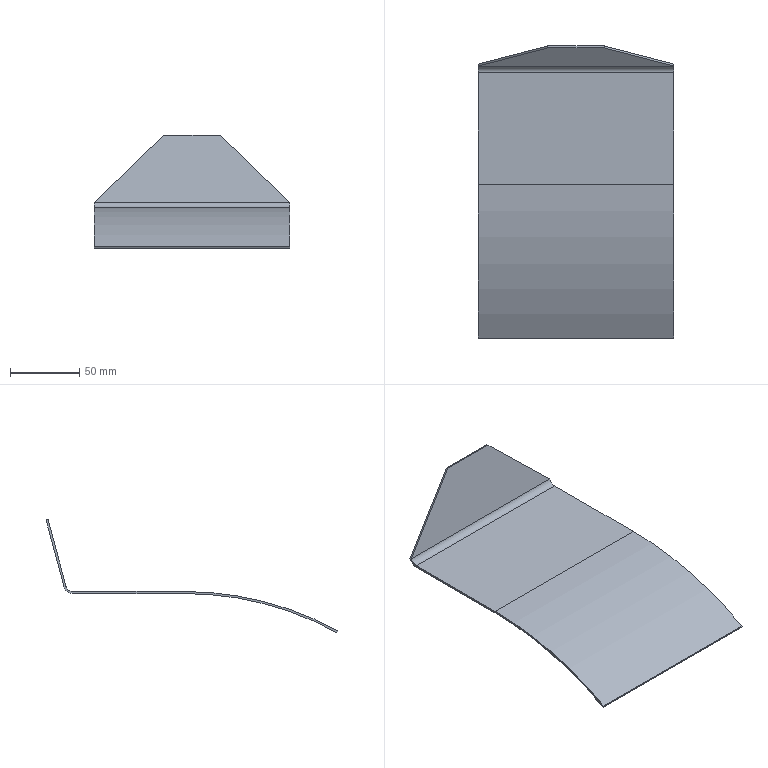Part | SolidWorks | features Chamfer 1, Extrusion 1 | 1 solid | 14 faces | box 141 x 210.455 x 81.673 mm | volume 49794 mm3 | plane 10 | cylinder 4 | commonest cylinder face diameters 10 x1 13 x1 458.6 x1 461.6 x1
STEP:
#1=CARTESIAN_POINT('',(-70.5,80.4,230.8));
#2=VERTEX_POINT('',#1);
#3=CARTESIAN_POINT('',(-70.5,85.23,234.506));
#4=VERTEX_POINT('',#3);
#5=CARTESIAN_POINT('',(-70.5,80.4,235.8));
#6=DIRECTION('',(1.,0.,0.));
#7=DIRECTION('',(0.,0.,-1.));
#8=AXIS2_PLACEMENT_3D('',#5,#6,#7);
#9=CIRCLE('',#8,5.);
#10=EDGE_CURVE('',#2,#4,#9,.T.);
#11=ORIENTED_EDGE('',*,*,#10,.F.);
#12=CARTESIAN_POINT('',(70.5,80.4,230.8));
#13=VERTEX_POINT('',#12);
#14=CARTESIAN_POINT('',(70.5,80.4,230.8));
#15=DIRECTION('',(-1.,0.,0.));
#16=VECTOR('',#15,1000.);
#17=LINE('',#14,#16);
#18=EDGE_CURVE('',#13,#2,#17,.T.);
#19=ORIENTED_EDGE('',*,*,#18,.F.);
#20=CARTESIAN_POINT('',(70.5,85.23,234.506));
#21=VERTEX_POINT('',#20);
#22=CARTESIAN_POINT('',(70.5,80.4,235.8));
#23=DIRECTION('',(1.,0.,0.));
#24=DIRECTION('',(0.,0.,-1.));
#25=AXIS2_PLACEMENT_3D('',#22,#23,#24);
#26=CIRCLE('',#25,5.);
#27=EDGE_CURVE('',#13,#21,#26,.T.);
#28=ORIENTED_EDGE('',*,*,#27,.T.);
#29=CARTESIAN_POINT('',(70.5,85.23,234.506));
#30=DIRECTION('',(-1.,0.,0.));
#31=VECTOR('',#30,1000.);
#32=LINE('',#29,#31);
#33=EDGE_CURVE('',#21,#4,#32,.T.);
#34=ORIENTED_EDGE('',*,*,#33,.T.);
#35=EDGE_LOOP('',(#11,#19,#28,#34));
#36=FACE_OUTER_BOUND('',#35,.T.);
#37=CARTESIAN_POINT('',(70.5,80.4,235.8));
#38=DIRECTION('',(-1.,0.,0.));
#39=DIRECTION('',(0.,0.,1.));
#40=AXIS2_PLACEMENT_3D('',#37,#38,#39);
#41=CYLINDRICAL_SURFACE('',#40,5.);
#42=ADVANCED_FACE('',(#36),#41,.F.);
#43=CARTESIAN_POINT('',(-70.5,0.,230.8));
#44=VERTEX_POINT('',#43);
#45=CARTESIAN_POINT('',(-70.5,0.,230.8));
#46=DIRECTION('',(0.,-1.,0.));
#47=VECTOR('',#46,1000.);
#48=LINE('',#45,#47);
#49=EDGE_CURVE('',#2,#44,#48,.T.);
#50=ORIENTED_EDGE('',*,*,#49,.T.);
#51=CARTESIAN_POINT('',(70.5,0.,230.8));
#52=VERTEX_POINT('',#51);
#53=CARTESIAN_POINT('',(70.5,0.,230.8));
#54=DIRECTION('',(-1.,0.,0.));
#55=VECTOR('',#54,1000.);
#56=LINE('',#53,#55);
#57=EDGE_CURVE('',#52,#44,#56,.T.);
#58=ORIENTED_EDGE('',*,*,#57,.F.);
#59=CARTESIAN_POINT('',(70.5,0.,230.8));
#60=DIRECTION('',(0.,-1.,0.));
#61=VECTOR('',#60,1000.);
#62=LINE('',#59,#61);
#63=EDGE_CURVE('',#13,#52,#62,.T.);
#64=ORIENTED_EDGE('',*,*,#63,.F.);
#65=ORIENTED_EDGE('',*,*,#18,.T.);
#66=EDGE_LOOP('',(#50,#58,#64,#65));
#67=FACE_OUTER_BOUND('',#66,.T.);
#68=CARTESIAN_POINT('',(70.5,0.,230.8));
#69=DIRECTION('',(0.,0.,-1.));
#70=DIRECTION('',(-1.,0.,0.));
#71=AXIS2_PLACEMENT_3D('',#68,#69,#70);
#72=PLANE('',#71);
#73=ADVANCED_FACE('',(#67),#72,.F.);
#74=CARTESIAN_POINT('',(-70.5,-110.836,202.445));
#75=VERTEX_POINT('',#74);
#76=CARTESIAN_POINT('',(-70.5,0.,0.));
#77=DIRECTION('',(1.,0.,0.));
#78=DIRECTION('',(0.,0.,-1.));
#79=AXIS2_PLACEMENT_3D('',#76,#77,#78);
#80=CIRCLE('',#79,230.8);
#81=EDGE_CURVE('',#44,#75,#80,.T.);
#82=ORIENTED_EDGE('',*,*,#81,.T.);
#83=CARTESIAN_POINT('',(70.5,-110.836,202.445));
#84=VERTEX_POINT('',#83);
#85=CARTESIAN_POINT('',(70.5,-110.836,202.445));
#86=DIRECTION('',(-1.,0.,0.));
#87=VECTOR('',#86,1000.);
#88=LINE('',#85,#87);
#89=EDGE_CURVE('',#84,#75,#88,.T.);
#90=ORIENTED_EDGE('',*,*,#89,.F.);
#91=CARTESIAN_POINT('',(70.5,0.,0.));
#92=DIRECTION('',(1.,0.,0.));
#93=DIRECTION('',(0.,0.,-1.));
#94=AXIS2_PLACEMENT_3D('',#91,#92,#93);
#95=CIRCLE('',#94,230.8);
#96=EDGE_CURVE('',#52,#84,#95,.T.);
#97=ORIENTED_EDGE('',*,*,#96,.F.);
#98=ORIENTED_EDGE('',*,*,#57,.T.);
#99=EDGE_LOOP('',(#82,#90,#97,#98));
#100=FACE_OUTER_BOUND('',#99,.T.);
#101=CARTESIAN_POINT('',(70.5,0.,0.));
#102=DIRECTION('',(-1.,0.,0.));
#103=DIRECTION('',(0.,0.,1.));
#104=AXIS2_PLACEMENT_3D('',#101,#102,#103);
#105=CYLINDRICAL_SURFACE('',#104,230.8);
#106=ADVANCED_FACE('',(#100),#105,.T.);
#107=CARTESIAN_POINT('',(-70.5,-110.115,201.13));
#108=VERTEX_POINT('',#107);
#109=CARTESIAN_POINT('',(-70.5,0.,0.));
#110=DIRECTION('',(0.,-0.4802,0.8771));
#111=VECTOR('',#110,1000.);
#112=LINE('',#109,#111);
#113=EDGE_CURVE('',#108,#75,#112,.T.);
#114=ORIENTED_EDGE('',*,*,#113,.F.);
#115=CARTESIAN_POINT('',(70.5,-110.115,201.13));
#116=VERTEX_POINT('',#115);
#117=CARTESIAN_POINT('',(70.5,-110.115,201.13));
#118=DIRECTION('',(-1.,0.,0.));
#119=VECTOR('',#118,1000.);
#120=LINE('',#117,#119);
#121=EDGE_CURVE('',#116,#108,#120,.T.);
#122=ORIENTED_EDGE('',*,*,#121,.F.);
#123=CARTESIAN_POINT('',(70.5,0.,0.));
#124=DIRECTION('',(0.,-0.4802,0.8771));
#125=VECTOR('',#124,1000.);
#126=LINE('',#123,#125);
#127=EDGE_CURVE('',#116,#84,#126,.T.);
#128=ORIENTED_EDGE('',*,*,#127,.T.);
#129=ORIENTED_EDGE('',*,*,#89,.T.);
#130=EDGE_LOOP('',(#114,#122,#128,#129));
#131=FACE_OUTER_BOUND('',#130,.T.);
#132=CARTESIAN_POINT('',(70.5,0.,0.));
#133=DIRECTION('',(0.,-0.8771,-0.4802));
#134=DIRECTION('',(0.,0.4802,-0.8771));
#135=AXIS2_PLACEMENT_3D('',#132,#133,#134);
#136=PLANE('',#135);
#137=ADVANCED_FACE('',(#131),#136,.T.);
#138=CARTESIAN_POINT('',(-70.5,0.,229.3));
#139=VERTEX_POINT('',#138);
#140=CARTESIAN_POINT('',(-70.5,0.,0.));
#141=DIRECTION('',(1.,0.,0.));
#142=DIRECTION('',(0.,0.,-1.));
#143=AXIS2_PLACEMENT_3D('',#140,#141,#142);
#144=CIRCLE('',#143,229.3);
#145=EDGE_CURVE('',#139,#108,#144,.T.);
#146=ORIENTED_EDGE('',*,*,#145,.F.);
#147=CARTESIAN_POINT('',(70.5,0.,229.3));
#148=VERTEX_POINT('',#147);
#149=CARTESIAN_POINT('',(70.5,0.,229.3));
#150=DIRECTION('',(-1.,0.,0.));
#151=VECTOR('',#150,1000.);
#152=LINE('',#149,#151);
#153=EDGE_CURVE('',#148,#139,#152,.T.);
#154=ORIENTED_EDGE('',*,*,#153,.F.);
#155=CARTESIAN_POINT('',(70.5,0.,0.));
#156=DIRECTION('',(1.,0.,0.));
#157=DIRECTION('',(0.,0.,-1.));
#158=AXIS2_PLACEMENT_3D('',#155,#156,#157);
#159=CIRCLE('',#158,229.3);
#160=EDGE_CURVE('',#148,#116,#159,.T.);
#161=ORIENTED_EDGE('',*,*,#160,.T.);
#162=ORIENTED_EDGE('',*,*,#121,.T.);
#163=EDGE_LOOP('',(#146,#154,#161,#162));
#164=FACE_OUTER_BOUND('',#163,.T.);
#165=CARTESIAN_POINT('',(70.5,0.,0.));
#166=DIRECTION('',(-1.,0.,0.));
#167=DIRECTION('',(0.,0.,1.));
#168=AXIS2_PLACEMENT_3D('',#165,#166,#167);
#169=CYLINDRICAL_SURFACE('',#168,229.3);
#170=ADVANCED_FACE('',(#164),#169,.F.);
#171=CARTESIAN_POINT('',(-70.5,80.4,229.3));
#172=VERTEX_POINT('',#171);
#173=CARTESIAN_POINT('',(-70.5,0.,229.3));
#174=DIRECTION('',(0.,1.,0.));
#175=VECTOR('',#174,1000.);
#176=LINE('',#173,#175);
#177=EDGE_CURVE('',#139,#172,#176,.T.);
#178=ORIENTED_EDGE('',*,*,#177,.T.);
#179=CARTESIAN_POINT('',(70.5,80.4,229.3));
#180=VERTEX_POINT('',#179);
#181=CARTESIAN_POINT('',(70.5,80.4,229.3));
#182=DIRECTION('',(-1.,0.,0.));
#183=VECTOR('',#182,1000.);
#184=LINE('',#181,#183);
#185=EDGE_CURVE('',#180,#172,#184,.T.);
#186=ORIENTED_EDGE('',*,*,#185,.F.);
#187=CARTESIAN_POINT('',(70.5,0.,229.3));
#188=DIRECTION('',(0.,1.,0.));
#189=VECTOR('',#188,1000.);
#190=LINE('',#187,#189);
#191=EDGE_CURVE('',#148,#180,#190,.T.);
#192=ORIENTED_EDGE('',*,*,#191,.F.);
#193=ORIENTED_EDGE('',*,*,#153,.T.);
#194=EDGE_LOOP('',(#178,#186,#192,#193));
#195=FACE_OUTER_BOUND('',#194,.T.);
#196=CARTESIAN_POINT('',(70.5,0.,229.3));
#197=DIRECTION('',(0.,0.,1.));
#198=DIRECTION('',(1.,0.,0.));
#199=AXIS2_PLACEMENT_3D('',#196,#197,#198);
#200=PLANE('',#199);
#201=ADVANCED_FACE('',(#195),#200,.F.);
#202=CARTESIAN_POINT('',(-70.5,86.679,234.118));
#203=VERTEX_POINT('',#202);
#204=CARTESIAN_POINT('',(-70.5,80.4,235.8));
#205=DIRECTION('',(1.,0.,0.));
#206=DIRECTION('',(0.,0.,-1.));
#207=AXIS2_PLACEMENT_3D('',#204,#205,#206);
#208=CIRCLE('',#207,6.5);
#209=EDGE_CURVE('',#172,#203,#208,.T.);
#210=ORIENTED_EDGE('',*,*,#209,.T.);
#211=CARTESIAN_POINT('',(70.5,86.679,234.118));
#212=VERTEX_POINT('',#211);
#213=CARTESIAN_POINT('',(70.5,86.679,234.118));
#214=DIRECTION('',(-1.,0.,0.));
#215=VECTOR('',#214,1000.);
#216=LINE('',#213,#215);
#217=EDGE_CURVE('',#212,#203,#216,.T.);
#218=ORIENTED_EDGE('',*,*,#217,.F.);
#219=CARTESIAN_POINT('',(70.5,80.4,235.8));
#220=DIRECTION('',(1.,0.,0.));
#221=DIRECTION('',(0.,0.,-1.));
#222=AXIS2_PLACEMENT_3D('',#219,#220,#221);
#223=CIRCLE('',#222,6.5);
#224=EDGE_CURVE('',#180,#212,#223,.T.);
#225=ORIENTED_EDGE('',*,*,#224,.F.);
#226=ORIENTED_EDGE('',*,*,#185,.T.);
#227=EDGE_LOOP('',(#210,#218,#225,#226));
#228=FACE_OUTER_BOUND('',#227,.T.);
#229=CARTESIAN_POINT('',(70.5,80.4,235.8));
#230=DIRECTION('',(-1.,0.,0.));
#231=DIRECTION('',(0.,0.,1.));
#232=AXIS2_PLACEMENT_3D('',#229,#230,#231);
#233=CYLINDRICAL_SURFACE('',#232,6.5);
#234=ADVANCED_FACE('',(#228),#233,.T.);
#235=ORIENTED_EDGE('',*,*,#217,.T.);
#236=CARTESIAN_POINT('',(-20.5,99.619,282.414));
#237=VERTEX_POINT('',#236);
#238=CARTESIAN_POINT('',(-20.5,99.619,282.414));
#239=DIRECTION('',(0.7071,0.183,0.683));
#240=VECTOR('',#239,1000.);
#241=LINE('',#238,#240);
#242=EDGE_CURVE('',#203,#237,#241,.T.);
#243=ORIENTED_EDGE('',*,*,#242,.T.);
#244=CARTESIAN_POINT('',(20.5,99.619,282.414));
#245=VERTEX_POINT('',#244);
#246=CARTESIAN_POINT('',(70.5,99.619,282.414));
#247=DIRECTION('',(-1.,0.,0.));
#248=VECTOR('',#247,1000.);
#249=LINE('',#246,#248);
#250=EDGE_CURVE('',#245,#237,#249,.T.);
#251=ORIENTED_EDGE('',*,*,#250,.F.);
#252=CARTESIAN_POINT('',(70.5,86.679,234.118));
#253=DIRECTION('',(0.7071,-0.183,-0.683));
#254=VECTOR('',#253,1000.);
#255=LINE('',#252,#254);
#256=EDGE_CURVE('',#245,#212,#255,.T.);
#257=ORIENTED_EDGE('',*,*,#256,.T.);
#258=EDGE_LOOP('',(#235,#243,#251,#257));
#259=FACE_OUTER_BOUND('',#258,.T.);
#260=CARTESIAN_POINT('',(70.5,22.343,-5.987));
#261=DIRECTION('',(0.,-0.9659,0.2588));
#262=DIRECTION('',(0.,-0.2588,-0.9659));
#263=AXIS2_PLACEMENT_3D('',#260,#261,#262);
#264=PLANE('',#263);
#265=ADVANCED_FACE('',(#259),#264,.F.);
#266=ORIENTED_EDGE('',*,*,#250,.T.);
#267=CARTESIAN_POINT('',(-20.5,98.171,282.802));
#268=VERTEX_POINT('',#267);
#269=CARTESIAN_POINT('',(-20.5,77.277,288.401));
#270=DIRECTION('',(0.,-0.9659,0.2588));
#271=VECTOR('',#270,1000.);
#272=LINE('',#269,#271);
#273=EDGE_CURVE('',#237,#268,#272,.T.);
#274=ORIENTED_EDGE('',*,*,#273,.T.);
#275=CARTESIAN_POINT('',(20.5,98.171,282.802));
#276=VERTEX_POINT('',#275);
#277=CARTESIAN_POINT('',(70.5,98.171,282.802));
#278=DIRECTION('',(-1.,0.,0.));
#279=VECTOR('',#278,1000.);
#280=LINE('',#277,#279);
#281=EDGE_CURVE('',#276,#268,#280,.T.);
#282=ORIENTED_EDGE('',*,*,#281,.F.);
#283=CARTESIAN_POINT('',(20.5,99.619,282.414));
#284=DIRECTION('',(0.,0.9659,-0.2588));
#285=VECTOR('',#284,1000.);
#286=LINE('',#283,#285);
#287=EDGE_CURVE('',#276,#245,#286,.T.);
#288=ORIENTED_EDGE('',*,*,#287,.T.);
#289=EDGE_LOOP('',(#266,#274,#282,#288));
#290=FACE_OUTER_BOUND('',#289,.T.);
#291=CARTESIAN_POINT('',(70.5,77.277,288.401));
#292=DIRECTION('',(0.,-0.2588,-0.9659));
#293=DIRECTION('',(0.,0.9659,-0.2588));
#294=AXIS2_PLACEMENT_3D('',#291,#292,#293);
#295=PLANE('',#294);
#296=ADVANCED_FACE('',(#290),#295,.F.);
#297=ORIENTED_EDGE('',*,*,#281,.T.);
#298=CARTESIAN_POINT('',(-20.5,98.171,282.802));
#299=DIRECTION('',(-0.7071,-0.183,-0.683));
#300=VECTOR('',#299,1000.);
#301=LINE('',#298,#300);
#302=EDGE_CURVE('',#268,#4,#301,.T.);
#303=ORIENTED_EDGE('',*,*,#302,.T.);
#304=ORIENTED_EDGE('',*,*,#33,.F.);
#305=CARTESIAN_POINT('',(70.5,85.23,234.506));
#306=DIRECTION('',(-0.7071,0.183,0.683));
#307=VECTOR('',#306,1000.);
#308=LINE('',#305,#307);
#309=EDGE_CURVE('',#21,#276,#308,.T.);
#310=ORIENTED_EDGE('',*,*,#309,.T.);
#311=EDGE_LOOP('',(#297,#303,#304,#310));
#312=FACE_OUTER_BOUND('',#311,.T.);
#313=CARTESIAN_POINT('',(70.5,20.894,-5.598));
#314=DIRECTION('',(0.,0.9659,-0.2588));
#315=DIRECTION('',(0.,0.2588,0.9659));
#316=AXIS2_PLACEMENT_3D('',#313,#314,#315);
#317=PLANE('',#316);
#318=ADVANCED_FACE('',(#312),#317,.F.);
#319=ORIENTED_EDGE('',*,*,#224,.T.);
#320=CARTESIAN_POINT('',(70.5,85.23,234.506));
#321=DIRECTION('',(0.,-0.9659,0.2588));
#322=VECTOR('',#321,1000.);
#323=LINE('',#320,#322);
#324=EDGE_CURVE('',#212,#21,#323,.T.);
#325=ORIENTED_EDGE('',*,*,#324,.T.);
#326=ORIENTED_EDGE('',*,*,#27,.F.);
#327=ORIENTED_EDGE('',*,*,#63,.T.);
#328=ORIENTED_EDGE('',*,*,#96,.T.);
#329=ORIENTED_EDGE('',*,*,#127,.F.);
#330=ORIENTED_EDGE('',*,*,#160,.F.);
#331=ORIENTED_EDGE('',*,*,#191,.T.);
#332=EDGE_LOOP('',(#319,#325,#326,#327,#328,#329,#330,#331));
#333=FACE_OUTER_BOUND('',#332,.T.);
#334=CARTESIAN_POINT('',(70.5,0.,0.));
#335=DIRECTION('',(1.,0.,0.));
#336=DIRECTION('',(0.,0.,-1.));
#337=AXIS2_PLACEMENT_3D('',#334,#335,#336);
#338=PLANE('',#337);
#339=ADVANCED_FACE('',(#333),#338,.T.);
#340=ORIENTED_EDGE('',*,*,#10,.T.);
#341=CARTESIAN_POINT('',(-70.5,64.336,240.104));
#342=DIRECTION('',(0.,0.9659,-0.2588));
#343=VECTOR('',#342,1000.);
#344=LINE('',#341,#343);
#345=EDGE_CURVE('',#4,#203,#344,.T.);
#346=ORIENTED_EDGE('',*,*,#345,.T.);
#347=ORIENTED_EDGE('',*,*,#209,.F.);
#348=ORIENTED_EDGE('',*,*,#177,.F.);
#349=ORIENTED_EDGE('',*,*,#145,.T.);
#350=ORIENTED_EDGE('',*,*,#113,.T.);
#351=ORIENTED_EDGE('',*,*,#81,.F.);
#352=ORIENTED_EDGE('',*,*,#49,.F.);
#353=EDGE_LOOP('',(#340,#346,#347,#348,#349,#350,#351,#352));
#354=FACE_OUTER_BOUND('',#353,.T.);
#355=CARTESIAN_POINT('',(-70.5,0.,0.));
#356=DIRECTION('',(1.,0.,0.));
#357=DIRECTION('',(0.,0.,-1.));
#358=AXIS2_PLACEMENT_3D('',#355,#356,#357);
#359=PLANE('',#358);
#360=ADVANCED_FACE('',(#354),#359,.F.);
#361=ORIENTED_EDGE('',*,*,#242,.F.);
#362=ORIENTED_EDGE('',*,*,#345,.F.);
#363=ORIENTED_EDGE('',*,*,#302,.F.);
#364=ORIENTED_EDGE('',*,*,#273,.F.);
#365=EDGE_LOOP('',(#361,#362,#363,#364));
#366=FACE_OUTER_BOUND('',#365,.T.);
#367=CARTESIAN_POINT('',(-20.5,77.277,288.401));
#368=DIRECTION('',(0.7071,-0.183,-0.683));
#369=DIRECTION('',(0.,-0.9659,0.2588));
#370=AXIS2_PLACEMENT_3D('',#367,#368,#369);
#371=PLANE('',#370);
#372=ADVANCED_FACE('',(#366),#371,.F.);
#373=ORIENTED_EDGE('',*,*,#256,.F.);
#374=ORIENTED_EDGE('',*,*,#287,.F.);
#375=ORIENTED_EDGE('',*,*,#309,.F.);
#376=ORIENTED_EDGE('',*,*,#324,.F.);
#377=EDGE_LOOP('',(#373,#374,#375,#376));
#378=FACE_OUTER_BOUND('',#377,.T.);
#379=CARTESIAN_POINT('',(70.5,64.336,240.104));
#380=DIRECTION('',(0.7071,0.183,0.683));
#381=DIRECTION('',(0.,0.9659,-0.2588));
#382=AXIS2_PLACEMENT_3D('',#379,#380,#381);
#383=PLANE('',#382);
#384=ADVANCED_FACE('',(#378),#383,.T.);
#385=CLOSED_SHELL('',(#42,#73,#106,#137,#170,#201,#234,#265,#296,#318,#339,#360,#372,#384));
#386=MANIFOLD_SOLID_BREP('',#385);
#387=CARTESIAN_POINT('',(0.,0.,0.));
#388=DIRECTION('',(0.,0.,1.));
#389=DIRECTION('',(1.,0.,0.));
#390=AXIS2_PLACEMENT_3D('',#387,#388,#389);
#391=(LENGTH_UNIT()NAMED_UNIT(*)SI_UNIT(.MILLI.,.METRE.));
#392=UNCERTAINTY_MEASURE_WITH_UNIT(LENGTH_MEASURE(0.00001),#391,'','');
#393=(NAMED_UNIT(*)PLANE_ANGLE_UNIT()SI_UNIT($,.RADIAN.));
#394=(NAMED_UNIT(*)SI_UNIT($,.STERADIAN.)SOLID_ANGLE_UNIT());
#395=(GEOMETRIC_REPRESENTATION_CONTEXT(3)GLOBAL_UNCERTAINTY_ASSIGNED_CONTEXT((#392))GLOBAL_UNIT_ASSIGNED_CONTEXT((#391,#393,#394))REPRESENTATION_CONTEXT('',''));
#396=ADVANCED_BREP_SHAPE_REPRESENTATION('',(#386,#390),#395);